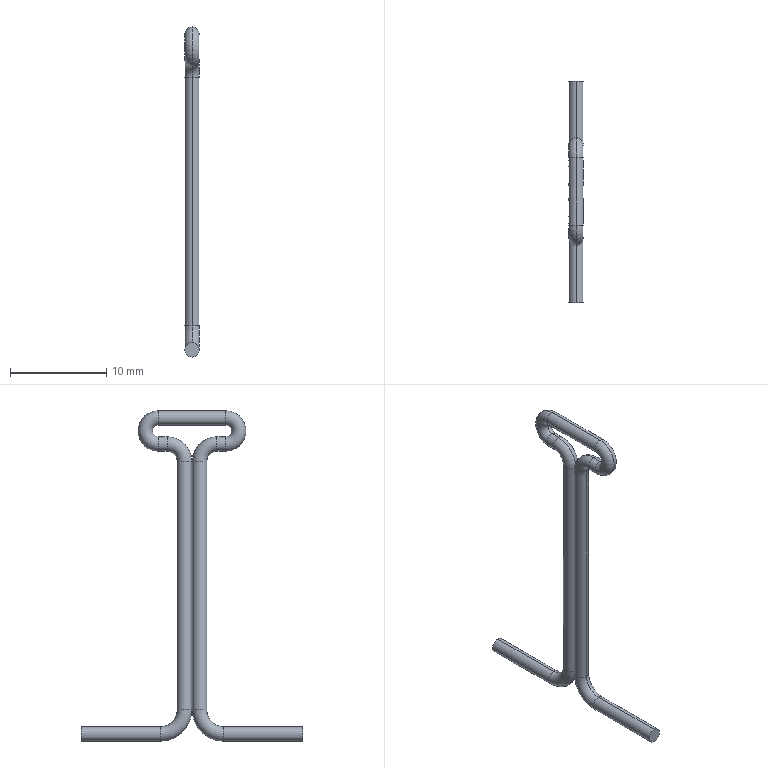Part | STEP file | Completa.sldasm-Part-107_Valor predeterminado | 1 solid | 28 faces | box 1.5 x 23 x 34.303 mm | volume 174.703 mm3 | cylinder 14 | torus 12 | plane 2 | commonest cylinder face diameters 1.5 x14